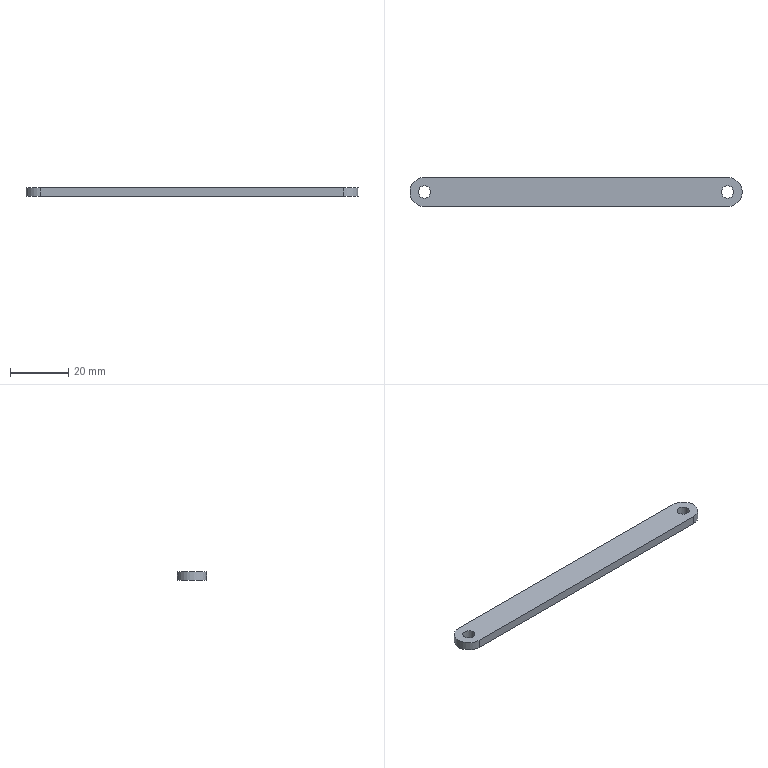Part | NX | features DATUM_CSYS 2, OFFSET_REGION 2, BREP 1, EXTRUDE 1, SCALE 1, SKETCH 1 | 1 solid | 8 faces | box 114 x 10 x 3 mm | volume 3272 mm3 | cylinder 4 | plane 4 | commonest cylinder face diameters 4.2 x2 10 x2
STEP:
#1=CARTESIAN_POINT('',(-214.239,-97.989,-2.5));
#2=VERTEX_POINT('',#1);
#3=CARTESIAN_POINT('',(-214.239,-107.989,-2.5));
#4=VERTEX_POINT('',#3);
#5=CARTESIAN_POINT('',(-214.239,-102.989,-2.5));
#6=DIRECTION('',(0.,0.,1.));
#7=DIRECTION('',(1.,0.,0.));
#8=AXIS2_PLACEMENT_3D('',#5,#6,#7);
#9=CIRCLE('',#8,5.);
#10=EDGE_CURVE('',#2,#4,#9,.T.);
#11=ORIENTED_EDGE('',*,*,#10,.F.);
#12=CARTESIAN_POINT('',(-214.239,-97.989,-5.5));
#13=VERTEX_POINT('',#12);
#14=CARTESIAN_POINT('',(-214.239,-97.989,-4.5));
#15=DIRECTION('',(0.,0.,-1.));
#16=VECTOR('',#15,1000.);
#17=LINE('',#14,#16);
#18=EDGE_CURVE('',#2,#13,#17,.T.);
#19=ORIENTED_EDGE('',*,*,#18,.T.);
#20=CARTESIAN_POINT('',(-214.239,-107.989,-5.5));
#21=VERTEX_POINT('',#20);
#22=CARTESIAN_POINT('',(-214.239,-102.989,-5.5));
#23=DIRECTION('',(0.,0.,1.));
#24=DIRECTION('',(1.,0.,0.));
#25=AXIS2_PLACEMENT_3D('',#22,#23,#24);
#26=CIRCLE('',#25,5.);
#27=EDGE_CURVE('',#13,#21,#26,.T.);
#28=ORIENTED_EDGE('',*,*,#27,.T.);
#29=CARTESIAN_POINT('',(-214.239,-107.989,-4.5));
#30=DIRECTION('',(0.,0.,1.));
#31=VECTOR('',#30,1000.);
#32=LINE('',#29,#31);
#33=EDGE_CURVE('',#4,#21,#32,.F.);
#34=ORIENTED_EDGE('',*,*,#33,.F.);
#35=EDGE_LOOP('',(#11,#19,#28,#34));
#36=FACE_BOUND('',#35,.T.);
#37=CARTESIAN_POINT('',(-214.239,-102.989,-4.5));
#38=DIRECTION('',(0.,0.,-1.));
#39=DIRECTION('',(-1.,0.,0.));
#40=AXIS2_PLACEMENT_3D('',#37,#38,#39);
#41=CYLINDRICAL_SURFACE('',#40,5.);
#42=ADVANCED_FACE('',(#36),#41,.T.);
#43=CARTESIAN_POINT('',(-110.239,-97.989,-5.5));
#44=VERTEX_POINT('',#43);
#45=CARTESIAN_POINT('',(-214.239,-97.989,-5.5));
#46=DIRECTION('',(1.,0.,0.));
#47=VECTOR('',#46,1000.);
#48=LINE('',#45,#47);
#49=EDGE_CURVE('',#13,#44,#48,.T.);
#50=ORIENTED_EDGE('',*,*,#49,.F.);
#51=ORIENTED_EDGE('',*,*,#18,.F.);
#52=CARTESIAN_POINT('',(-110.239,-97.989,-2.5));
#53=VERTEX_POINT('',#52);
#54=CARTESIAN_POINT('',(-214.239,-97.989,-2.5));
#55=DIRECTION('',(1.,0.,0.));
#56=VECTOR('',#55,1000.);
#57=LINE('',#54,#56);
#58=EDGE_CURVE('',#2,#53,#57,.T.);
#59=ORIENTED_EDGE('',*,*,#58,.T.);
#60=CARTESIAN_POINT('',(-110.239,-97.989,-4.5));
#61=DIRECTION('',(0.,0.,1.));
#62=VECTOR('',#61,1000.);
#63=LINE('',#60,#62);
#64=EDGE_CURVE('',#53,#44,#63,.F.);
#65=ORIENTED_EDGE('',*,*,#64,.T.);
#66=EDGE_LOOP('',(#50,#51,#59,#65));
#67=FACE_BOUND('',#66,.T.);
#68=CARTESIAN_POINT('',(-214.239,-97.989,-4.5));
#69=DIRECTION('',(0.,1.,0.));
#70=DIRECTION('',(-1.,0.,0.));
#71=AXIS2_PLACEMENT_3D('',#68,#69,#70);
#72=PLANE('',#71);
#73=ADVANCED_FACE('',(#67),#72,.T.);
#74=CARTESIAN_POINT('',(-110.239,-107.989,-5.5));
#75=VERTEX_POINT('',#74);
#76=CARTESIAN_POINT('',(-214.239,-107.989,-5.5));
#77=DIRECTION('',(1.,0.,0.));
#78=VECTOR('',#77,1000.);
#79=LINE('',#76,#78);
#80=EDGE_CURVE('',#21,#75,#79,.T.);
#81=ORIENTED_EDGE('',*,*,#80,.T.);
#82=CARTESIAN_POINT('',(-110.239,-107.989,-2.5));
#83=VERTEX_POINT('',#82);
#84=CARTESIAN_POINT('',(-110.239,-107.989,-4.5));
#85=DIRECTION('',(0.,0.,-1.));
#86=VECTOR('',#85,1000.);
#87=LINE('',#84,#86);
#88=EDGE_CURVE('',#83,#75,#87,.T.);
#89=ORIENTED_EDGE('',*,*,#88,.F.);
#90=CARTESIAN_POINT('',(-214.239,-107.989,-2.5));
#91=DIRECTION('',(1.,0.,0.));
#92=VECTOR('',#91,1000.);
#93=LINE('',#90,#92);
#94=EDGE_CURVE('',#4,#83,#93,.T.);
#95=ORIENTED_EDGE('',*,*,#94,.F.);
#96=ORIENTED_EDGE('',*,*,#33,.T.);
#97=EDGE_LOOP('',(#81,#89,#95,#96));
#98=FACE_BOUND('',#97,.T.);
#99=CARTESIAN_POINT('',(-214.239,-107.989,-4.5));
#100=DIRECTION('',(0.,1.,0.));
#101=DIRECTION('',(-1.,0.,0.));
#102=AXIS2_PLACEMENT_3D('',#99,#100,#101);
#103=PLANE('',#102);
#104=ADVANCED_FACE('',(#98),#103,.F.);
#105=CARTESIAN_POINT('',(-110.239,-102.989,-5.5));
#106=DIRECTION('',(0.,0.,1.));
#107=DIRECTION('',(1.,0.,0.));
#108=AXIS2_PLACEMENT_3D('',#105,#106,#107);
#109=CIRCLE('',#108,5.);
#110=EDGE_CURVE('',#75,#44,#109,.T.);
#111=ORIENTED_EDGE('',*,*,#110,.T.);
#112=ORIENTED_EDGE('',*,*,#64,.F.);
#113=CARTESIAN_POINT('',(-110.239,-102.989,-2.5));
#114=DIRECTION('',(0.,0.,1.));
#115=DIRECTION('',(1.,0.,0.));
#116=AXIS2_PLACEMENT_3D('',#113,#114,#115);
#117=CIRCLE('',#116,5.);
#118=EDGE_CURVE('',#83,#53,#117,.T.);
#119=ORIENTED_EDGE('',*,*,#118,.F.);
#120=ORIENTED_EDGE('',*,*,#88,.T.);
#121=EDGE_LOOP('',(#111,#112,#119,#120));
#122=FACE_BOUND('',#121,.T.);
#123=CARTESIAN_POINT('',(-110.239,-102.989,-4.5));
#124=DIRECTION('',(0.,0.,-1.));
#125=DIRECTION('',(-1.,0.,0.));
#126=AXIS2_PLACEMENT_3D('',#123,#124,#125);
#127=CYLINDRICAL_SURFACE('',#126,5.);
#128=ADVANCED_FACE('',(#122),#127,.T.);
#129=CARTESIAN_POINT('',(-108.139,-102.989,-2.5));
#130=VERTEX_POINT('',#129);
#131=CARTESIAN_POINT('',(-110.239,-102.989,-2.5));
#132=DIRECTION('',(0.,0.,1.));
#133=DIRECTION('',(1.,0.,0.));
#134=AXIS2_PLACEMENT_3D('',#131,#132,#133);
#135=CIRCLE('',#134,2.1);
#136=EDGE_CURVE('',#130,#130,#135,.F.);
#137=ORIENTED_EDGE('',*,*,#136,.T.);
#138=EDGE_LOOP('',(#137));
#139=FACE_BOUND('',#138,.T.);
#140=CARTESIAN_POINT('',(-212.139,-102.989,-2.5));
#141=VERTEX_POINT('',#140);
#142=CARTESIAN_POINT('',(-214.239,-102.989,-2.5));
#143=DIRECTION('',(0.,0.,1.));
#144=DIRECTION('',(1.,0.,0.));
#145=AXIS2_PLACEMENT_3D('',#142,#143,#144);
#146=CIRCLE('',#145,2.1);
#147=EDGE_CURVE('',#141,#141,#146,.F.);
#148=ORIENTED_EDGE('',*,*,#147,.T.);
#149=EDGE_LOOP('',(#148));
#150=FACE_BOUND('',#149,.T.);
#151=ORIENTED_EDGE('',*,*,#58,.F.);
#152=ORIENTED_EDGE('',*,*,#10,.T.);
#153=ORIENTED_EDGE('',*,*,#94,.T.);
#154=ORIENTED_EDGE('',*,*,#118,.T.);
#155=EDGE_LOOP('',(#151,#152,#153,#154));
#156=FACE_BOUND('',#155,.T.);
#157=CARTESIAN_POINT('',(-110.239,-102.989,-2.5));
#158=DIRECTION('',(0.,0.,1.));
#159=DIRECTION('',(1.,0.,0.));
#160=AXIS2_PLACEMENT_3D('',#157,#158,#159);
#161=PLANE('',#160);
#162=ADVANCED_FACE('',(#139,#150,#156),#161,.T.);
#163=CARTESIAN_POINT('',(-108.139,-102.989,-5.5));
#164=VERTEX_POINT('',#163);
#165=CARTESIAN_POINT('',(-110.239,-102.989,-5.5));
#166=DIRECTION('',(0.,0.,1.));
#167=DIRECTION('',(1.,0.,0.));
#168=AXIS2_PLACEMENT_3D('',#165,#166,#167);
#169=CIRCLE('',#168,2.1);
#170=EDGE_CURVE('',#164,#164,#169,.F.);
#171=ORIENTED_EDGE('',*,*,#170,.F.);
#172=EDGE_LOOP('',(#171));
#173=FACE_BOUND('',#172,.T.);
#174=CARTESIAN_POINT('',(-212.139,-102.989,-5.5));
#175=VERTEX_POINT('',#174);
#176=CARTESIAN_POINT('',(-214.239,-102.989,-5.5));
#177=DIRECTION('',(0.,0.,1.));
#178=DIRECTION('',(1.,0.,0.));
#179=AXIS2_PLACEMENT_3D('',#176,#177,#178);
#180=CIRCLE('',#179,2.1);
#181=EDGE_CURVE('',#175,#175,#180,.F.);
#182=ORIENTED_EDGE('',*,*,#181,.F.);
#183=EDGE_LOOP('',(#182));
#184=FACE_BOUND('',#183,.T.);
#185=ORIENTED_EDGE('',*,*,#49,.T.);
#186=ORIENTED_EDGE('',*,*,#110,.F.);
#187=ORIENTED_EDGE('',*,*,#80,.F.);
#188=ORIENTED_EDGE('',*,*,#27,.F.);
#189=EDGE_LOOP('',(#185,#186,#187,#188));
#190=FACE_BOUND('',#189,.T.);
#191=CARTESIAN_POINT('',(-110.239,-102.989,-5.5));
#192=DIRECTION('',(0.,0.,1.));
#193=DIRECTION('',(1.,0.,0.));
#194=AXIS2_PLACEMENT_3D('',#191,#192,#193);
#195=PLANE('',#194);
#196=ADVANCED_FACE('',(#173,#184,#190),#195,.F.);
#197=ORIENTED_EDGE('',*,*,#147,.F.);
#198=EDGE_LOOP('',(#197));
#199=FACE_BOUND('',#198,.T.);
#200=ORIENTED_EDGE('',*,*,#181,.T.);
#201=EDGE_LOOP('',(#200));
#202=FACE_BOUND('',#201,.T.);
#203=CARTESIAN_POINT('',(-214.239,-102.989,0.5));
#204=DIRECTION('',(0.,0.,-1.));
#205=DIRECTION('',(-1.,0.,0.));
#206=AXIS2_PLACEMENT_3D('',#203,#204,#205);
#207=CYLINDRICAL_SURFACE('',#206,2.1);
#208=ADVANCED_FACE('',(#199,#202),#207,.F.);
#209=ORIENTED_EDGE('',*,*,#136,.F.);
#210=EDGE_LOOP('',(#209));
#211=FACE_BOUND('',#210,.T.);
#212=ORIENTED_EDGE('',*,*,#170,.T.);
#213=EDGE_LOOP('',(#212));
#214=FACE_BOUND('',#213,.T.);
#215=CARTESIAN_POINT('',(-110.239,-102.989,0.5));
#216=DIRECTION('',(0.,0.,-1.));
#217=DIRECTION('',(-1.,0.,0.));
#218=AXIS2_PLACEMENT_3D('',#215,#216,#217);
#219=CYLINDRICAL_SURFACE('',#218,2.1);
#220=ADVANCED_FACE('',(#211,#214),#219,.F.);
#221=CLOSED_SHELL('',(#42,#73,#104,#128,#162,#196,#208,#220));
#222=MANIFOLD_SOLID_BREP('',#221);
#223=(LENGTH_UNIT()NAMED_UNIT(*)SI_UNIT(.MILLI.,.METRE.));
#224=UNCERTAINTY_MEASURE_WITH_UNIT(LENGTH_MEASURE(0.00001),#223,'','');
#225=(NAMED_UNIT(*)PLANE_ANGLE_UNIT()SI_UNIT($,.RADIAN.));
#226=(NAMED_UNIT(*)SI_UNIT($,.STERADIAN.)SOLID_ANGLE_UNIT());
#227=(GEOMETRIC_REPRESENTATION_CONTEXT(3)GLOBAL_UNCERTAINTY_ASSIGNED_CONTEXT((#224))GLOBAL_UNIT_ASSIGNED_CONTEXT((#223,#225,#226))REPRESENTATION_CONTEXT('',''));
#228=ADVANCED_BREP_SHAPE_REPRESENTATION('',(#222),#227);